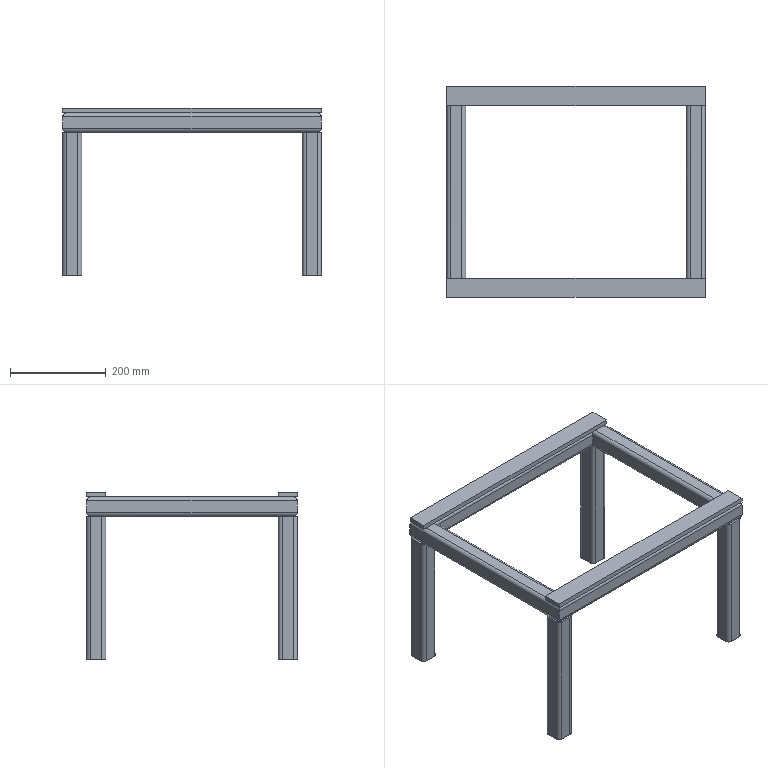Part | SolidWorks | features 3DProfileFeature 1, ICE 1, MirrorSolid 1, WeldMemberFeat 1, WeldmentFeature 1 | 10 solids | 156 faces | box 540 x 440 x 350 mm | volume 2036389 mm3 | plane 92 | cylinder 64 | commonest cylinder face diameters 8 x32 16 x32